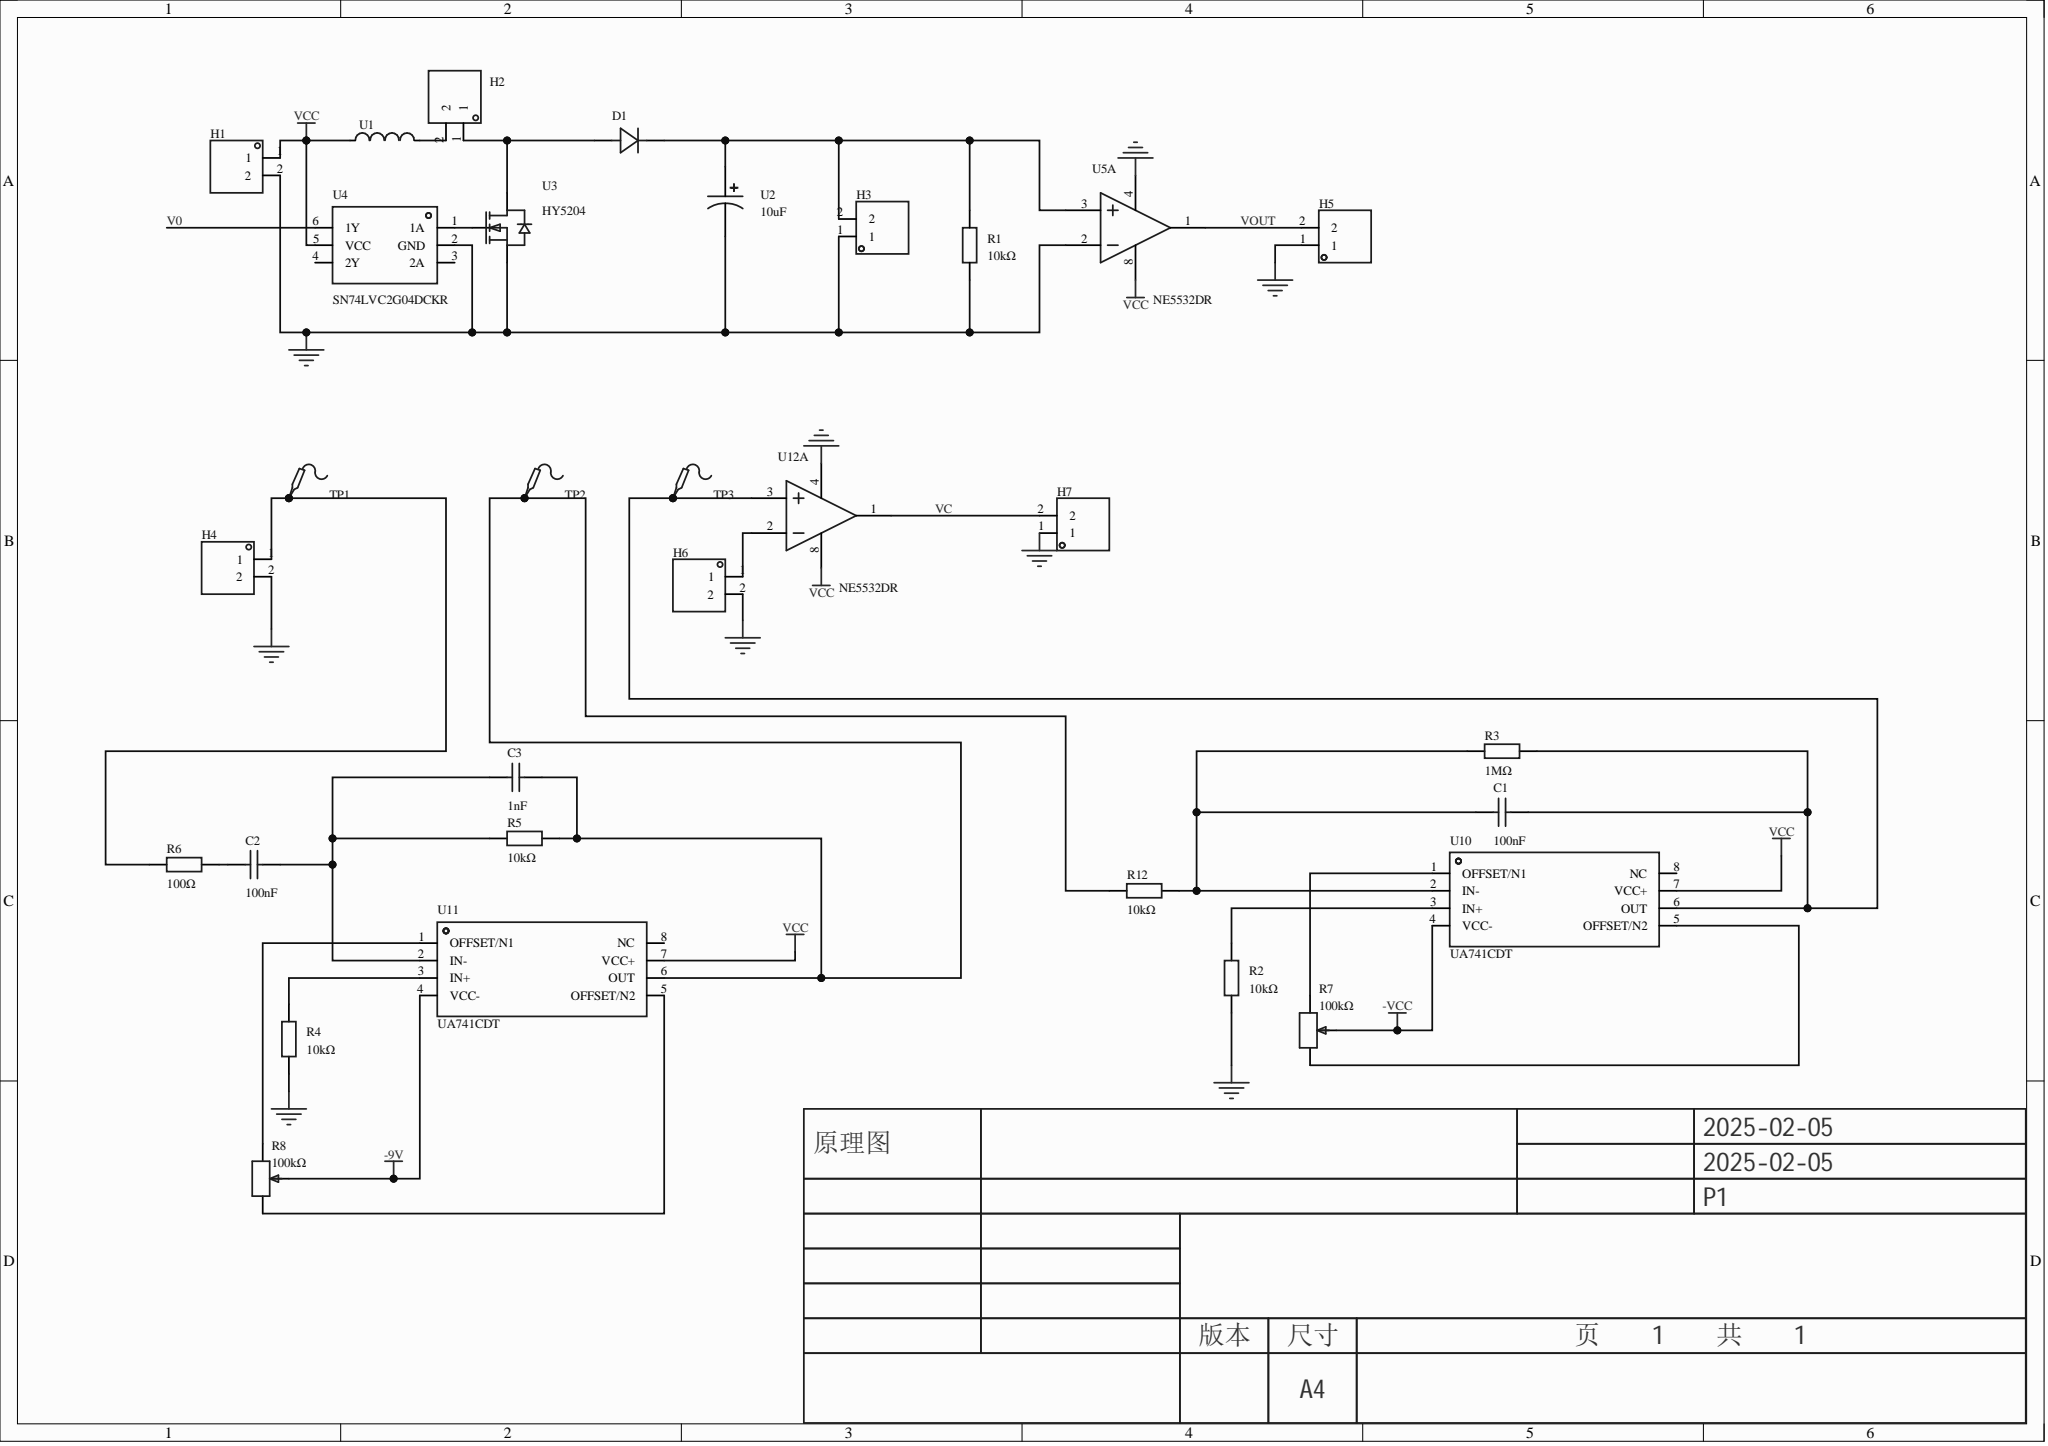Circuit board | Altium Designer | 31 parts | 23 nets
Bill of materials:
Comment,Description,Designator,Footprint,LibRef,Quantity
"100nF","","C1, C2","C0805","CC0805KRX7R9BB104","2"
"1nF","","C3","C0805","CC0805KRX7R9BB104","1"
"","","D1","DO_1N4007","D_1N4007A","1"
"","","H1, H2, H3, H4, H5, H6, H7","HDR-TH_2P-P2.54-V-M-1","HDR-M_2.54_1x2P","7"
"10kΩ","","R1","Res_1/4W","Res_AXIAL-1/4W","1"
"10kΩ","","R2, R4, R5, R12","R0805","0805W8F1002T5E_C17414","4"
"1MΩ","","R3","R0805","0805W8F1002T5E_C17414","1"
"100Ω","","R6","R0805","0805W8F1002T5E_C17414","1"
"100kΩ","","R7, R8","RES-ADJ-SMD_VG039NCH","VG039NCHXTB201","2"
"","","TP1, TP2, TP3","Test-Point-0.5mm","Test-Point","3"
"功率电感(贴片),CKST0502-10uH/M,10uH,±20%,3A,封装5.7mm*5.1mm*2.0mm,岑科,RoHS","","U1","IND-SMD_L5.7-W5.1","功率电感(贴片),CKST0502-10uH/M,10uH,±20%,3A,封装5.7mm*5.1mm*2.0mm,岑科,RoHS","1"
"10uF","","U2","CAP-TH_BD4.0-P1.50-D0.8-FD","10MS510MEFC4X5","1"
"HY5204","","U3","TO-247-3_L15.8-W5.0-P5.44-L-1","HY5204","1"
"SN74LVC2G04DCKR","","U4","SOT-363_L2.0-W1.3-P0.65-LS2.1-BR","SN74LVC2G04DCKR","1"
"NE5532DR","","U5, U12","SOIC-8_L4.9-W3.9-P1.27-LS6.0-BL","NE5532DR","2"
"UA741CDT","","U10, U11","SOIC-8_L4.9-W3.9-P1.27-LS6.0-BL","UA741CDT","2"
Netlist (Protel format):
[
C1
C0805
100nF



]
[
C2
C0805
100nF



]
[
C3
C0805
1nF



]
[
D1
DO_1N4007




]
[
H1
HDR-TH_2P-P2.54-V-M-1




]
[
H2
HDR-TH_2P-P2.54-V-M-1




]
[
H3
HDR-TH_2P-P2.54-V-M-1




]
[
H4
HDR-TH_2P-P2.54-V-M-1




]
[
H5
HDR-TH_2P-P2.54-V-M-1




]
[
H6
HDR-TH_2P-P2.54-V-M-1




]
[
H7
HDR-TH_2P-P2.54-V-M-1




]
[
R1
Res_1/4W
10kΩ



]
[
R2
R0805
10kΩ



]
[
R3
R0805
1MΩ



]
[
R4
R0805
10kΩ



]
[
R5
R0805
10kΩ



]
[
R6
R0805
100Ω



]
[
R7
RES-ADJ-SMD_VG039NCH
100kΩ



]
[
R8
RES-ADJ-SMD_VG039NCH
100kΩ



]
[
R12
R0805
10kΩ



]
[
TP1
Test-Point-0.5mm




]
[
TP2
Test-Point-0.5mm




]
[
TP3
Test-Point-0.5mm




]
[
U1
IND-SMD_L5.7-W5.1
功率电感(贴片),CKST0502-10uH/M,10uH,±20%,3A,封装5.7mm*5.1mm*2.0mm,岑科,RoHS



]
[
U2
CAP-TH_BD4.0-P1.50-D0.8-FD
10uF



]
[
U3
TO-247-3_L15.8-W5.0-P5.44-L-1
HY5204



]
[
U4
SOT-363_L2.0-W1.3-P0.65-LS2.1-BR
SN74LVC2G04DCKR



]
[
U5
SOIC-8_L4.9-W3.9-P1.27-LS6.0-BL
NE5532DR



]
[
U10
SOIC-8_L4.9-W3.9-P1.27-LS6.0-BL
UA741CDT



]
[
U11
SOIC-8_L4.9-W3.9-P1.27-LS6.0-BL
UA741CDT



]
[
U12
SOIC-8_L4.9-W3.9-P1.27-LS6.0-BL
NE5532DR



]
(
VOUT
H5-2
U5-1
)
(
VCC
H1-1
U1-1
U4-5
U5-8
U10-7
U11-7
U12-8
)
(
VC
H7-2
U12-1
)
(
NetU3_1
U3-1
U4-1
)
(
NetR8_3
R8-3
U11-5
)
(
NetR8_1
R8-1
U11-1
)
(
NetR7_3
R7-3
U10-1
)
(
NetR7_1
R7-1
U10-5
)
(
NetR4_2
R4-2
U11-3
)
(
NetR2_2
R2-2
U10-3
)
(
NetH6_1
H6-1
U12-2
)
(
NetH4_1
H4-1
R6-1
TP1-1
)
(
NetH2_2
H2-2
U1-2
)
(
NetD1_2
D1-2
H2-1
U3-2
)
(
NetD1_1
D1-1
H3-2
R1-2
U2-1
U5-3
)
(
NetC3_2
C3-2
R5-2
R12-1
TP2-1
U11-6
)
(
NetC2_2
C2-2
C3-1
R5-1
U11-2
)
(
NetC2_1
C2-1
R6-2
)
(
NetC1_2
C1-2
R3-2
TP3-1
U10-6
U12-3
)
(
NetC1_1
C1-1
R3-1
R12-2
U10-2
)
(
GND
H1-2
H3-1
H4-2
H5-1
H6-2
H7-1
R1-1
R2-1
R4-1
U2-2
U3-3
U4-2
U5-2
U5-4
U12-4
)
(
-VCC
R7-2
U10-4
)
(
-9V
R8-2
U11-4
)